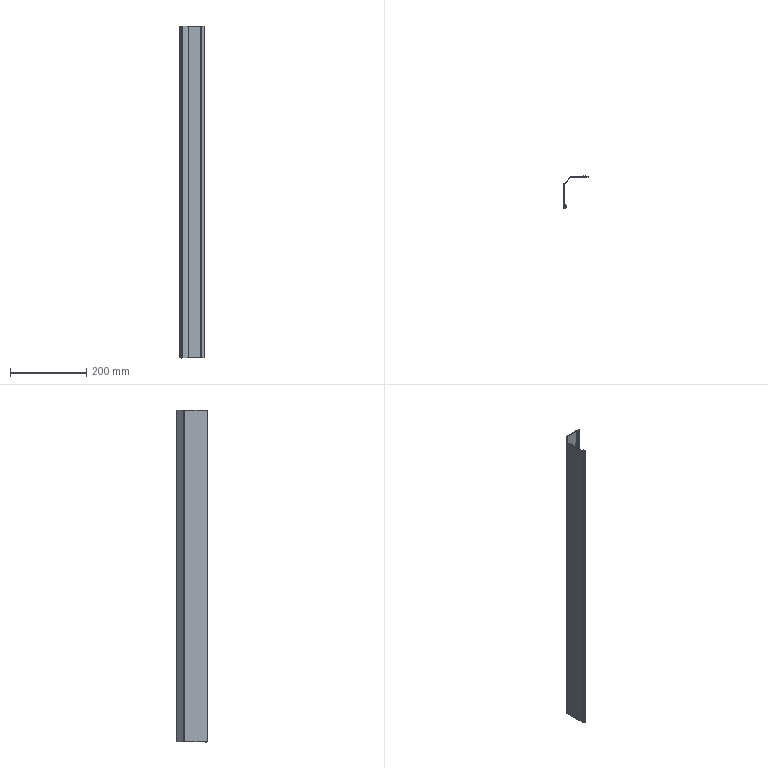Part | STEP file | 51E-01208JG10 | 1 solid | 53 faces | box 65 x 82.9 x 870 mm | volume 179523 mm3 | cylinder 30 | plane 23 | commonest cylinder face diameters 1 x9 1.8 x6 0.9 x4 0.4 x3 0.6 x2 3 x2